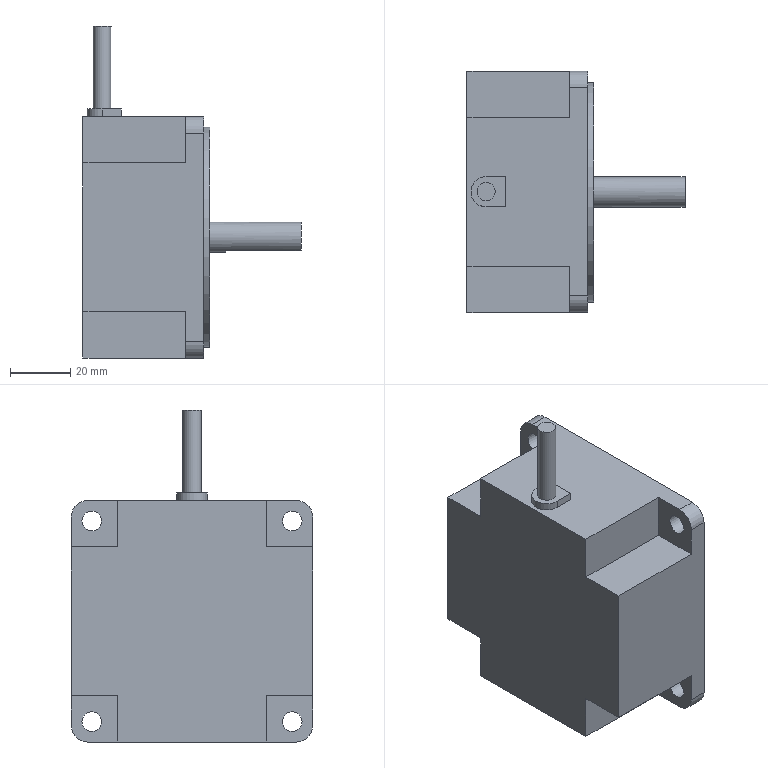Part | NX | features 5003_108_Stepper motor 2 | 1 solid | 41 faces | box 72.25 x 80 x 110 mm | volume 229003 mm3 | plane 28 | cylinder 13 | commonest cylinder face diameters 6.5 x4 11 x4 10 x2 6 x1 35 x1 73 x1
STEP:
#1=CARTESIAN_POINT('',(-49.115,60.,-76.5));
#2=VERTEX_POINT('',#1);
#3=CARTESIAN_POINT('',(-55.415,60.,-76.5));
#4=VERTEX_POINT('',#3);
#5=CARTESIAN_POINT('',(-49.115,60.,-76.5));
#6=DIRECTION('',(-1.,0.,0.));
#7=VECTOR('',#6,1000.);
#8=LINE('',#5,#7);
#9=EDGE_CURVE('',#2,#4,#8,.T.);
#10=ORIENTED_EDGE('',*,*,#9,.T.);
#11=CARTESIAN_POINT('',(-55.415,50.,-76.5));
#12=VERTEX_POINT('',#11);
#13=CARTESIAN_POINT('',(-55.415,55.,-76.5));
#14=DIRECTION('',(0.,0.,1.));
#15=DIRECTION('',(0.,-1.,0.));
#16=AXIS2_PLACEMENT_3D('',#13,#14,#15);
#17=CIRCLE('',#16,5.);
#18=EDGE_CURVE('',#4,#12,#17,.T.);
#19=ORIENTED_EDGE('',*,*,#18,.T.);
#20=CARTESIAN_POINT('',(-49.115,50.,-76.5));
#21=VERTEX_POINT('',#20);
#22=CARTESIAN_POINT('',(-49.115,50.,-76.5));
#23=DIRECTION('',(1.,0.,0.));
#24=VECTOR('',#23,1000.);
#25=LINE('',#22,#24);
#26=EDGE_CURVE('',#12,#21,#25,.T.);
#27=ORIENTED_EDGE('',*,*,#26,.T.);
#28=CARTESIAN_POINT('',(-49.115,60.,-76.5));
#29=DIRECTION('',(0.,1.,0.));
#30=VECTOR('',#29,1000.);
#31=LINE('',#28,#30);
#32=EDGE_CURVE('',#21,#2,#31,.T.);
#33=ORIENTED_EDGE('',*,*,#32,.T.);
#34=EDGE_LOOP('',(#10,#19,#27,#33));
#35=FACE_BOUND('',#34,.T.);
#36=CARTESIAN_POINT('',(-55.415,52.,-76.5));
#37=VERTEX_POINT('',#36);
#38=CARTESIAN_POINT('',(-55.415,55.,-76.5));
#39=DIRECTION('',(0.,0.,1.));
#40=DIRECTION('',(0.,-1.,0.));
#41=AXIS2_PLACEMENT_3D('',#38,#39,#40);
#42=CIRCLE('',#41,3.);
#43=EDGE_CURVE('',#37,#37,#42,.T.);
#44=ORIENTED_EDGE('',*,*,#43,.F.);
#45=EDGE_LOOP('',(#44));
#46=FACE_BOUND('',#45,.T.);
#47=CARTESIAN_POINT('',(-55.415,55.,-76.5));
#48=DIRECTION('',(0.,0.,1.));
#49=DIRECTION('',(0.,-1.,0.));
#50=AXIS2_PLACEMENT_3D('',#47,#48,#49);
#51=PLANE('',#50);
#52=ADVANCED_FACE('',(#35,#46),#51,.T.);
#53=CARTESIAN_POINT('',(-27.725,20.5,-79.));
#54=VERTEX_POINT('',#53);
#55=CARTESIAN_POINT('',(-21.725,20.5,-79.));
#56=VERTEX_POINT('',#55);
#57=CARTESIAN_POINT('',(-61.725,20.5,-79.));
#58=DIRECTION('',(1.,0.,0.));
#59=VECTOR('',#58,1000.);
#60=LINE('',#57,#59);
#61=EDGE_CURVE('',#54,#56,#60,.T.);
#62=ORIENTED_EDGE('',*,*,#61,.T.);
#63=CARTESIAN_POINT('',(-21.725,89.5,-79.));
#64=VERTEX_POINT('',#63);
#65=CARTESIAN_POINT('',(-21.725,95.,-79.));
#66=DIRECTION('',(0.,1.,0.));
#67=VECTOR('',#66,1000.);
#68=LINE('',#65,#67);
#69=EDGE_CURVE('',#56,#64,#68,.T.);
#70=ORIENTED_EDGE('',*,*,#69,.T.);
#71=CARTESIAN_POINT('',(-27.725,89.5,-79.));
#72=VERTEX_POINT('',#71);
#73=CARTESIAN_POINT('',(-61.725,89.5,-79.));
#74=DIRECTION('',(1.,0.,0.));
#75=VECTOR('',#74,1000.);
#76=LINE('',#73,#75);
#77=EDGE_CURVE('',#64,#72,#76,.F.);
#78=ORIENTED_EDGE('',*,*,#77,.T.);
#79=CARTESIAN_POINT('',(-27.725,79.65,-79.));
#80=VERTEX_POINT('',#79);
#81=CARTESIAN_POINT('',(-27.725,95.,-79.));
#82=DIRECTION('',(0.,-1.,0.));
#83=VECTOR('',#82,1000.);
#84=LINE('',#81,#83);
#85=EDGE_CURVE('',#72,#80,#84,.T.);
#86=ORIENTED_EDGE('',*,*,#85,.T.);
#87=CARTESIAN_POINT('',(-61.725,79.65,-79.));
#88=VERTEX_POINT('',#87);
#89=CARTESIAN_POINT('',(-27.725,79.65,-79.));
#90=DIRECTION('',(-1.,0.,0.));
#91=VECTOR('',#90,1000.);
#92=LINE('',#89,#91);
#93=EDGE_CURVE('',#80,#88,#92,.T.);
#94=ORIENTED_EDGE('',*,*,#93,.T.);
#95=CARTESIAN_POINT('',(-61.725,30.35,-79.));
#96=VERTEX_POINT('',#95);
#97=CARTESIAN_POINT('',(-61.725,95.,-79.));
#98=DIRECTION('',(0.,-1.,0.));
#99=VECTOR('',#98,1000.);
#100=LINE('',#97,#99);
#101=EDGE_CURVE('',#88,#96,#100,.T.);
#102=ORIENTED_EDGE('',*,*,#101,.T.);
#103=CARTESIAN_POINT('',(-27.725,30.35,-79.));
#104=VERTEX_POINT('',#103);
#105=CARTESIAN_POINT('',(-27.725,30.35,-79.));
#106=DIRECTION('',(-1.,0.,0.));
#107=VECTOR('',#106,1000.);
#108=LINE('',#105,#107);
#109=EDGE_CURVE('',#104,#96,#108,.T.);
#110=ORIENTED_EDGE('',*,*,#109,.F.);
#111=CARTESIAN_POINT('',(-27.725,95.,-79.));
#112=DIRECTION('',(0.,-1.,0.));
#113=VECTOR('',#112,1000.);
#114=LINE('',#111,#113);
#115=EDGE_CURVE('',#104,#54,#114,.T.);
#116=ORIENTED_EDGE('',*,*,#115,.T.);
#117=EDGE_LOOP('',(#62,#70,#78,#86,#94,#102,#110,#116));
#118=FACE_BOUND('',#117,.T.);
#119=CARTESIAN_POINT('',(-55.415,60.,-79.));
#120=VERTEX_POINT('',#119);
#121=CARTESIAN_POINT('',(-55.415,50.,-79.));
#122=VERTEX_POINT('',#121);
#123=CARTESIAN_POINT('',(-55.415,55.,-79.));
#124=DIRECTION('',(0.,0.,1.));
#125=DIRECTION('',(0.,-1.,0.));
#126=AXIS2_PLACEMENT_3D('',#123,#124,#125);
#127=CIRCLE('',#126,5.);
#128=EDGE_CURVE('',#120,#122,#127,.T.);
#129=ORIENTED_EDGE('',*,*,#128,.F.);
#130=CARTESIAN_POINT('',(-49.115,60.,-79.));
#131=VERTEX_POINT('',#130);
#132=CARTESIAN_POINT('',(-49.115,60.,-79.));
#133=DIRECTION('',(-1.,0.,0.));
#134=VECTOR('',#133,1000.);
#135=LINE('',#132,#134);
#136=EDGE_CURVE('',#131,#120,#135,.T.);
#137=ORIENTED_EDGE('',*,*,#136,.F.);
#138=CARTESIAN_POINT('',(-49.115,50.,-79.));
#139=VERTEX_POINT('',#138);
#140=CARTESIAN_POINT('',(-49.115,60.,-79.));
#141=DIRECTION('',(0.,1.,0.));
#142=VECTOR('',#141,1000.);
#143=LINE('',#140,#142);
#144=EDGE_CURVE('',#139,#131,#143,.T.);
#145=ORIENTED_EDGE('',*,*,#144,.F.);
#146=CARTESIAN_POINT('',(-49.115,50.,-79.));
#147=DIRECTION('',(1.,0.,0.));
#148=VECTOR('',#147,1000.);
#149=LINE('',#146,#148);
#150=EDGE_CURVE('',#122,#139,#149,.T.);
#151=ORIENTED_EDGE('',*,*,#150,.F.);
#152=EDGE_LOOP('',(#129,#137,#145,#151));
#153=FACE_BOUND('',#152,.T.);
#154=CARTESIAN_POINT('',(-61.725,95.,-79.));
#155=DIRECTION('',(0.,0.,1.));
#156=DIRECTION('',(0.,-1.,0.));
#157=AXIS2_PLACEMENT_3D('',#154,#155,#156);
#158=PLANE('',#157);
#159=ADVANCED_FACE('',(#118,#153),#158,.T.);
#160=CARTESIAN_POINT('',(-26.225,37.5,-119.));
#161=VERTEX_POINT('',#160);
#162=CARTESIAN_POINT('',(-26.225,55.,-119.));
#163=DIRECTION('',(1.,0.,0.));
#164=DIRECTION('',(0.,-1.,0.));
#165=AXIS2_PLACEMENT_3D('',#162,#163,#164);
#166=CIRCLE('',#165,17.5);
#167=EDGE_CURVE('',#161,#161,#166,.T.);
#168=ORIENTED_EDGE('',*,*,#167,.T.);
#169=EDGE_LOOP('',(#168));
#170=FACE_BOUND('',#169,.T.);
#171=CARTESIAN_POINT('',(-26.225,50.,-119.));
#172=VERTEX_POINT('',#171);
#173=CARTESIAN_POINT('',(-26.225,55.,-119.));
#174=DIRECTION('',(1.,0.,0.));
#175=DIRECTION('',(0.,-1.,0.));
#176=AXIS2_PLACEMENT_3D('',#173,#174,#175);
#177=CIRCLE('',#176,5.);
#178=EDGE_CURVE('',#172,#172,#177,.T.);
#179=ORIENTED_EDGE('',*,*,#178,.F.);
#180=EDGE_LOOP('',(#179));
#181=FACE_BOUND('',#180,.T.);
#182=CARTESIAN_POINT('',(-26.225,55.,-119.));
#183=DIRECTION('',(1.,0.,0.));
#184=DIRECTION('',(0.,-1.,0.));
#185=AXIS2_PLACEMENT_3D('',#182,#183,#184);
#186=PLANE('',#185);
#187=ADVANCED_FACE('',(#170,#181),#186,.T.);
#188=CARTESIAN_POINT('',(-27.725,95.,-84.5));
#189=VERTEX_POINT('',#188);
#190=CARTESIAN_POINT('',(-21.725,95.,-84.5));
#191=VERTEX_POINT('',#190);
#192=CARTESIAN_POINT('',(-61.725,95.,-84.5));
#193=DIRECTION('',(1.,0.,0.));
#194=VECTOR('',#193,1000.);
#195=LINE('',#192,#194);
#196=EDGE_CURVE('',#189,#191,#195,.T.);
#197=ORIENTED_EDGE('',*,*,#196,.T.);
#198=CARTESIAN_POINT('',(-21.725,95.,-153.5));
#199=VERTEX_POINT('',#198);
#200=CARTESIAN_POINT('',(-21.725,95.,-159.));
#201=DIRECTION('',(0.,0.,-1.));
#202=VECTOR('',#201,1000.);
#203=LINE('',#200,#202);
#204=EDGE_CURVE('',#191,#199,#203,.T.);
#205=ORIENTED_EDGE('',*,*,#204,.T.);
#206=CARTESIAN_POINT('',(-27.725,95.,-153.5));
#207=VERTEX_POINT('',#206);
#208=CARTESIAN_POINT('',(-61.725,95.,-153.5));
#209=DIRECTION('',(1.,0.,0.));
#210=VECTOR('',#209,1000.);
#211=LINE('',#208,#210);
#212=EDGE_CURVE('',#199,#207,#211,.F.);
#213=ORIENTED_EDGE('',*,*,#212,.T.);
#214=CARTESIAN_POINT('',(-27.725,95.,-143.65));
#215=VERTEX_POINT('',#214);
#216=CARTESIAN_POINT('',(-27.725,95.,-159.));
#217=DIRECTION('',(0.,0.,1.));
#218=VECTOR('',#217,1000.);
#219=LINE('',#216,#218);
#220=EDGE_CURVE('',#207,#215,#219,.T.);
#221=ORIENTED_EDGE('',*,*,#220,.T.);
#222=CARTESIAN_POINT('',(-61.725,95.,-143.65));
#223=VERTEX_POINT('',#222);
#224=CARTESIAN_POINT('',(-27.725,95.,-143.65));
#225=DIRECTION('',(-1.,0.,0.));
#226=VECTOR('',#225,1000.);
#227=LINE('',#224,#226);
#228=EDGE_CURVE('',#215,#223,#227,.T.);
#229=ORIENTED_EDGE('',*,*,#228,.T.);
#230=CARTESIAN_POINT('',(-61.725,95.,-94.35));
#231=VERTEX_POINT('',#230);
#232=CARTESIAN_POINT('',(-61.725,95.,-159.));
#233=DIRECTION('',(0.,0.,1.));
#234=VECTOR('',#233,1000.);
#235=LINE('',#232,#234);
#236=EDGE_CURVE('',#223,#231,#235,.T.);
#237=ORIENTED_EDGE('',*,*,#236,.T.);
#238=CARTESIAN_POINT('',(-27.725,95.,-94.35));
#239=VERTEX_POINT('',#238);
#240=CARTESIAN_POINT('',(-27.725,95.,-94.35));
#241=DIRECTION('',(-1.,0.,0.));
#242=VECTOR('',#241,1000.);
#243=LINE('',#240,#242);
#244=EDGE_CURVE('',#239,#231,#243,.T.);
#245=ORIENTED_EDGE('',*,*,#244,.F.);
#246=CARTESIAN_POINT('',(-27.725,95.,-159.));
#247=DIRECTION('',(0.,0.,1.));
#248=VECTOR('',#247,1000.);
#249=LINE('',#246,#248);
#250=EDGE_CURVE('',#239,#189,#249,.T.);
#251=ORIENTED_EDGE('',*,*,#250,.T.);
#252=EDGE_LOOP('',(#197,#205,#213,#221,#229,#237,#245,#251));
#253=FACE_BOUND('',#252,.T.);
#254=CARTESIAN_POINT('',(-61.725,95.,-159.));
#255=DIRECTION('',(0.,1.,0.));
#256=DIRECTION('',(0.,0.,1.));
#257=AXIS2_PLACEMENT_3D('',#254,#255,#256);
#258=PLANE('',#257);
#259=ADVANCED_FACE('',(#253),#258,.T.);
#260=CARTESIAN_POINT('',(-27.725,89.5,-159.));
#261=VERTEX_POINT('',#260);
#262=CARTESIAN_POINT('',(-21.725,89.5,-159.));
#263=VERTEX_POINT('',#262);
#264=CARTESIAN_POINT('',(-61.725,89.5,-159.));
#265=DIRECTION('',(1.,0.,0.));
#266=VECTOR('',#265,1000.);
#267=LINE('',#264,#266);
#268=EDGE_CURVE('',#261,#263,#267,.T.);
#269=ORIENTED_EDGE('',*,*,#268,.T.);
#270=CARTESIAN_POINT('',(-21.725,20.5,-159.));
#271=VERTEX_POINT('',#270);
#272=CARTESIAN_POINT('',(-21.725,95.,-159.));
#273=DIRECTION('',(0.,-1.,0.));
#274=VECTOR('',#273,1000.);
#275=LINE('',#272,#274);
#276=EDGE_CURVE('',#263,#271,#275,.T.);
#277=ORIENTED_EDGE('',*,*,#276,.T.);
#278=CARTESIAN_POINT('',(-27.725,20.5,-159.));
#279=VERTEX_POINT('',#278);
#280=CARTESIAN_POINT('',(-61.725,20.5,-159.));
#281=DIRECTION('',(1.,0.,0.));
#282=VECTOR('',#281,1000.);
#283=LINE('',#280,#282);
#284=EDGE_CURVE('',#271,#279,#283,.F.);
#285=ORIENTED_EDGE('',*,*,#284,.T.);
#286=CARTESIAN_POINT('',(-27.725,30.35,-159.));
#287=VERTEX_POINT('',#286);
#288=CARTESIAN_POINT('',(-27.725,95.,-159.));
#289=DIRECTION('',(0.,1.,0.));
#290=VECTOR('',#289,1000.);
#291=LINE('',#288,#290);
#292=EDGE_CURVE('',#279,#287,#291,.T.);
#293=ORIENTED_EDGE('',*,*,#292,.T.);
#294=CARTESIAN_POINT('',(-61.725,30.35,-159.));
#295=VERTEX_POINT('',#294);
#296=CARTESIAN_POINT('',(-27.725,30.35,-159.));
#297=DIRECTION('',(-1.,0.,0.));
#298=VECTOR('',#297,1000.);
#299=LINE('',#296,#298);
#300=EDGE_CURVE('',#287,#295,#299,.T.);
#301=ORIENTED_EDGE('',*,*,#300,.T.);
#302=CARTESIAN_POINT('',(-61.725,79.65,-159.));
#303=VERTEX_POINT('',#302);
#304=CARTESIAN_POINT('',(-61.725,95.,-159.));
#305=DIRECTION('',(0.,1.,0.));
#306=VECTOR('',#305,1000.);
#307=LINE('',#304,#306);
#308=EDGE_CURVE('',#295,#303,#307,.T.);
#309=ORIENTED_EDGE('',*,*,#308,.T.);
#310=CARTESIAN_POINT('',(-27.725,79.65,-159.));
#311=VERTEX_POINT('',#310);
#312=CARTESIAN_POINT('',(-27.725,79.65,-159.));
#313=DIRECTION('',(-1.,0.,0.));
#314=VECTOR('',#313,1000.);
#315=LINE('',#312,#314);
#316=EDGE_CURVE('',#311,#303,#315,.T.);
#317=ORIENTED_EDGE('',*,*,#316,.F.);
#318=CARTESIAN_POINT('',(-27.725,95.,-159.));
#319=DIRECTION('',(0.,1.,0.));
#320=VECTOR('',#319,1000.);
#321=LINE('',#318,#320);
#322=EDGE_CURVE('',#311,#261,#321,.T.);
#323=ORIENTED_EDGE('',*,*,#322,.T.);
#324=EDGE_LOOP('',(#269,#277,#285,#293,#301,#309,#317,#323));
#325=FACE_BOUND('',#324,.T.);
#326=CARTESIAN_POINT('',(-61.725,95.,-159.));
#327=DIRECTION('',(0.,0.,-1.));
#328=DIRECTION('',(0.,1.,0.));
#329=AXIS2_PLACEMENT_3D('',#326,#327,#328);
#330=PLANE('',#329);
#331=ADVANCED_FACE('',(#325),#330,.T.);
#332=CARTESIAN_POINT('',(-27.725,15.,-153.5));
#333=VERTEX_POINT('',#332);
#334=CARTESIAN_POINT('',(-21.725,15.,-153.5));
#335=VERTEX_POINT('',#334);
#336=CARTESIAN_POINT('',(-61.725,15.,-153.5));
#337=DIRECTION('',(1.,0.,0.));
#338=VECTOR('',#337,1000.);
#339=LINE('',#336,#338);
#340=EDGE_CURVE('',#333,#335,#339,.T.);
#341=ORIENTED_EDGE('',*,*,#340,.T.);
#342=CARTESIAN_POINT('',(-21.725,15.,-84.5));
#343=VERTEX_POINT('',#342);
#344=CARTESIAN_POINT('',(-21.725,15.,-159.));
#345=DIRECTION('',(0.,0.,1.));
#346=VECTOR('',#345,1000.);
#347=LINE('',#344,#346);
#348=EDGE_CURVE('',#335,#343,#347,.T.);
#349=ORIENTED_EDGE('',*,*,#348,.T.);
#350=CARTESIAN_POINT('',(-27.725,15.,-84.5));
#351=VERTEX_POINT('',#350);
#352=CARTESIAN_POINT('',(-61.725,15.,-84.5));
#353=DIRECTION('',(1.,0.,0.));
#354=VECTOR('',#353,1000.);
#355=LINE('',#352,#354);
#356=EDGE_CURVE('',#343,#351,#355,.F.);
#357=ORIENTED_EDGE('',*,*,#356,.T.);
#358=CARTESIAN_POINT('',(-27.725,15.,-94.35));
#359=VERTEX_POINT('',#358);
#360=CARTESIAN_POINT('',(-27.725,15.,-159.));
#361=DIRECTION('',(0.,0.,-1.));
#362=VECTOR('',#361,1000.);
#363=LINE('',#360,#362);
#364=EDGE_CURVE('',#351,#359,#363,.T.);
#365=ORIENTED_EDGE('',*,*,#364,.T.);
#366=CARTESIAN_POINT('',(-61.725,15.,-94.35));
#367=VERTEX_POINT('',#366);
#368=CARTESIAN_POINT('',(-27.725,15.,-94.35));
#369=DIRECTION('',(-1.,0.,0.));
#370=VECTOR('',#369,1000.);
#371=LINE('',#368,#370);
#372=EDGE_CURVE('',#359,#367,#371,.T.);
#373=ORIENTED_EDGE('',*,*,#372,.T.);
#374=CARTESIAN_POINT('',(-61.725,15.,-143.65));
#375=VERTEX_POINT('',#374);
#376=CARTESIAN_POINT('',(-61.725,15.,-159.));
#377=DIRECTION('',(0.,0.,-1.));
#378=VECTOR('',#377,1000.);
#379=LINE('',#376,#378);
#380=EDGE_CURVE('',#367,#375,#379,.T.);
#381=ORIENTED_EDGE('',*,*,#380,.T.);
#382=CARTESIAN_POINT('',(-27.725,15.,-143.65));
#383=VERTEX_POINT('',#382);
#384=CARTESIAN_POINT('',(-27.725,15.,-143.65));
#385=DIRECTION('',(-1.,0.,0.));
#386=VECTOR('',#385,1000.);
#387=LINE('',#384,#386);
#388=EDGE_CURVE('',#383,#375,#387,.T.);
#389=ORIENTED_EDGE('',*,*,#388,.F.);
#390=CARTESIAN_POINT('',(-27.725,15.,-159.));
#391=DIRECTION('',(0.,0.,-1.));
#392=VECTOR('',#391,1000.);
#393=LINE('',#390,#392);
#394=EDGE_CURVE('',#383,#333,#393,.T.);
#395=ORIENTED_EDGE('',*,*,#394,.T.);
#396=EDGE_LOOP('',(#341,#349,#357,#365,#373,#381,#389,#395));
#397=FACE_BOUND('',#396,.T.);
#398=CARTESIAN_POINT('',(-61.725,15.,-159.));
#399=DIRECTION('',(0.,-1.,0.));
#400=DIRECTION('',(0.,0.,-1.));
#401=AXIS2_PLACEMENT_3D('',#398,#399,#400);
#402=PLANE('',#401);
#403=ADVANCED_FACE('',(#397),#402,.T.);
#404=ORIENTED_EDGE('',*,*,#356,.F.);
#405=CARTESIAN_POINT('',(-21.725,20.5,-84.5));
#406=DIRECTION('',(1.,0.,0.));
#407=DIRECTION('',(0.,-1.,0.));
#408=AXIS2_PLACEMENT_3D('',#405,#406,#407);
#409=CIRCLE('',#408,5.5);
#410=EDGE_CURVE('',#343,#56,#409,.F.);
#411=ORIENTED_EDGE('',*,*,#410,.T.);
#412=ORIENTED_EDGE('',*,*,#61,.F.);
#413=CARTESIAN_POINT('',(-27.725,20.5,-84.5));
#414=DIRECTION('',(-1.,0.,0.));
#415=DIRECTION('',(0.,1.,0.));
#416=AXIS2_PLACEMENT_3D('',#413,#414,#415);
#417=CIRCLE('',#416,5.5);
#418=EDGE_CURVE('',#351,#54,#417,.T.);
#419=ORIENTED_EDGE('',*,*,#418,.F.);
#420=EDGE_LOOP('',(#404,#411,#412,#419));
#421=FACE_BOUND('',#420,.T.);
#422=CARTESIAN_POINT('',(-61.725,20.5,-84.5));
#423=DIRECTION('',(1.,0.,0.));
#424=DIRECTION('',(0.,-1.,0.));
#425=AXIS2_PLACEMENT_3D('',#422,#423,#424);
#426=CYLINDRICAL_SURFACE('',#425,5.5);
#427=ADVANCED_FACE('',(#421),#426,.T.);
#428=ORIENTED_EDGE('',*,*,#77,.F.);
#429=CARTESIAN_POINT('',(-21.725,89.5,-84.5));
#430=DIRECTION('',(1.,0.,0.));
#431=DIRECTION('',(0.,-1.,0.));
#432=AXIS2_PLACEMENT_3D('',#429,#430,#431);
#433=CIRCLE('',#432,5.5);
#434=EDGE_CURVE('',#64,#191,#433,.F.);
#435=ORIENTED_EDGE('',*,*,#434,.T.);
#436=ORIENTED_EDGE('',*,*,#196,.F.);
#437=CARTESIAN_POINT('',(-27.725,89.5,-84.5));
#438=DIRECTION('',(-1.,0.,0.));
#439=DIRECTION('',(0.,1.,0.));
#440=AXIS2_PLACEMENT_3D('',#437,#438,#439);
#441=CIRCLE('',#440,5.5);
#442=EDGE_CURVE('',#72,#189,#441,.T.);
#443=ORIENTED_EDGE('',*,*,#442,.F.);
#444=EDGE_LOOP('',(#428,#435,#436,#443));
#445=FACE_BOUND('',#444,.T.);
#446=CARTESIAN_POINT('',(-61.725,89.5,-84.5));
#447=DIRECTION('',(1.,0.,0.));
#448=DIRECTION('',(0.,-1.,0.));
#449=AXIS2_PLACEMENT_3D('',#446,#447,#448);
#450=CYLINDRICAL_SURFACE('',#449,5.5);
#451=ADVANCED_FACE('',(#445),#450,.T.);
#452=ORIENTED_EDGE('',*,*,#212,.F.);
#453=CARTESIAN_POINT('',(-21.725,89.5,-153.5));
#454=DIRECTION('',(1.,0.,0.));
#455=DIRECTION('',(0.,-1.,0.));
#456=AXIS2_PLACEMENT_3D('',#453,#454,#455);
#457=CIRCLE('',#456,5.5);
#458=EDGE_CURVE('',#199,#263,#457,.F.);
#459=ORIENTED_EDGE('',*,*,#458,.T.);
#460=ORIENTED_EDGE('',*,*,#268,.F.);
#461=CARTESIAN_POINT('',(-27.725,89.5,-153.5));
#462=DIRECTION('',(-1.,0.,0.));
#463=DIRECTION('',(0.,1.,0.));
#464=AXIS2_PLACEMENT_3D('',#461,#462,#463);
#465=CIRCLE('',#464,5.5);
#466=EDGE_CURVE('',#207,#261,#465,.T.);
#467=ORIENTED_EDGE('',*,*,#466,.F.);
#468=EDGE_LOOP('',(#452,#459,#460,#467));
#469=FACE_BOUND('',#468,.T.);
#470=CARTESIAN_POINT('',(-61.725,89.5,-153.5));
#471=DIRECTION('',(1.,0.,0.));
#472=DIRECTION('',(0.,-1.,0.));
#473=AXIS2_PLACEMENT_3D('',#470,#471,#472);
#474=CYLINDRICAL_SURFACE('',#473,5.5);
#475=ADVANCED_FACE('',(#469),#474,.T.);
#476=ORIENTED_EDGE('',*,*,#284,.F.);
#477=CARTESIAN_POINT('',(-21.725,20.5,-153.5));
#478=DIRECTION('',(1.,0.,0.));
#479=DIRECTION('',(0.,-1.,0.));
#480=AXIS2_PLACEMENT_3D('',#477,#478,#479);
#481=CIRCLE('',#480,5.5);
#482=EDGE_CURVE('',#271,#335,#481,.F.);
#483=ORIENTED_EDGE('',*,*,#482,.T.);
#484=ORIENTED_EDGE('',*,*,#340,.F.);
#485=CARTESIAN_POINT('',(-27.725,20.5,-153.5));
#486=DIRECTION('',(-1.,0.,0.));
#487=DIRECTION('',(0.,1.,0.));
#488=AXIS2_PLACEMENT_3D('',#485,#486,#487);
#489=CIRCLE('',#488,5.5);
#490=EDGE_CURVE('',#279,#333,#489,.T.);
#491=ORIENTED_EDGE('',*,*,#490,.F.);
#492=EDGE_LOOP('',(#476,#483,#484,#491));
#493=FACE_BOUND('',#492,.T.);
#494=CARTESIAN_POINT('',(-61.725,20.5,-153.5));
#495=DIRECTION('',(1.,0.,0.));
#496=DIRECTION('',(0.,-1.,0.));
#497=AXIS2_PLACEMENT_3D('',#494,#495,#496);
#498=CYLINDRICAL_SURFACE('',#497,5.5);
#499=ADVANCED_FACE('',(#493),#498,.T.);
#500=CARTESIAN_POINT('',(-27.725,91.484,-85.766));
#501=VERTEX_POINT('',#500);
#502=CARTESIAN_POINT('',(-27.725,88.234,-85.766));
#503=DIRECTION('',(-1.,0.,0.));
#504=DIRECTION('',(0.,1.,0.));
#505=AXIS2_PLACEMENT_3D('',#502,#503,#504);
#506=CIRCLE('',#505,3.25);
#507=EDGE_CURVE('',#501,#501,#506,.T.);
#508=ORIENTED_EDGE('',*,*,#507,.T.);
#509=EDGE_LOOP('',(#508));
#510=FACE_BOUND('',#509,.T.);
#511=CARTESIAN_POINT('',(-21.725,84.984,-85.766));
#512=VERTEX_POINT('',#511);
#513=CARTESIAN_POINT('',(-21.725,88.234,-85.766));
#514=DIRECTION('',(1.,0.,0.));
#515=DIRECTION('',(0.,-1.,0.));
#516=AXIS2_PLACEMENT_3D('',#513,#514,#515);
#517=CIRCLE('',#516,3.25);
#518=EDGE_CURVE('',#512,#512,#517,.F.);
#519=ORIENTED_EDGE('',*,*,#518,.F.);
#520=EDGE_LOOP('',(#519));
#521=FACE_BOUND('',#520,.T.);
#522=CARTESIAN_POINT('',(-19.725,88.234,-85.766));
#523=DIRECTION('',(1.,0.,0.));
#524=DIRECTION('',(0.,-1.,0.));
#525=AXIS2_PLACEMENT_3D('',#522,#523,#524);
#526=CYLINDRICAL_SURFACE('',#525,3.25);
#527=ADVANCED_FACE('',(#510,#521),#526,.F.);
#528=CARTESIAN_POINT('',(-27.725,25.016,-85.766));
#529=VERTEX_POINT('',#528);
#530=CARTESIAN_POINT('',(-27.725,21.766,-85.766));
#531=DIRECTION('',(-1.,0.,0.));
#532=DIRECTION('',(0.,1.,0.));
#533=AXIS2_PLACEMENT_3D('',#530,#531,#532);
#534=CIRCLE('',#533,3.25);
#535=EDGE_CURVE('',#529,#529,#534,.T.);
#536=ORIENTED_EDGE('',*,*,#535,.T.);
#537=EDGE_LOOP('',(#536));
#538=FACE_BOUND('',#537,.T.);
#539=CARTESIAN_POINT('',(-21.725,18.516,-85.766));
#540=VERTEX_POINT('',#539);
#541=CARTESIAN_POINT('',(-21.725,21.766,-85.766));
#542=DIRECTION('',(1.,0.,0.));
#543=DIRECTION('',(0.,-1.,0.));
#544=AXIS2_PLACEMENT_3D('',#541,#542,#543);
#545=CIRCLE('',#544,3.25);
#546=EDGE_CURVE('',#540,#540,#545,.F.);
#547=ORIENTED_EDGE('',*,*,#546,.F.);
#548=EDGE_LOOP('',(#547));
#549=FACE_BOUND('',#548,.T.);
#550=CARTESIAN_POINT('',(-19.725,21.766,-85.766));
#551=DIRECTION('',(1.,0.,0.));
#552=DIRECTION('',(0.,-1.,0.));
#553=AXIS2_PLACEMENT_3D('',#550,#551,#552);
#554=CYLINDRICAL_SURFACE('',#553,3.25);
#555=ADVANCED_FACE('',(#538,#549),#554,.F.);
#556=CARTESIAN_POINT('',(-27.725,25.016,-152.234));
#557=VERTEX_POINT('',#556);
#558=CARTESIAN_POINT('',(-27.725,21.766,-152.234));
#559=DIRECTION('',(-1.,0.,0.));
#560=DIRECTION('',(0.,1.,0.));
#561=AXIS2_PLACEMENT_3D('',#558,#559,#560);
#562=CIRCLE('',#561,3.25);
#563=EDGE_CURVE('',#557,#557,#562,.T.);
#564=ORIENTED_EDGE('',*,*,#563,.T.);
#565=EDGE_LOOP('',(#564));
#566=FACE_BOUND('',#565,.T.);
#567=CARTESIAN_POINT('',(-21.725,18.516,-152.234));
#568=VERTEX_POINT('',#567);
#569=CARTESIAN_POINT('',(-21.725,21.766,-152.234));
#570=DIRECTION('',(1.,0.,0.));
#571=DIRECTION('',(0.,-1.,0.));
#572=AXIS2_PLACEMENT_3D('',#569,#570,#571);
#573=CIRCLE('',#572,3.25);
#574=EDGE_CURVE('',#568,#568,#573,.F.);
#575=ORIENTED_EDGE('',*,*,#574,.F.);
#576=EDGE_LOOP('',(#575));
#577=FACE_BOUND('',#576,.T.);
#578=CARTESIAN_POINT('',(-19.725,21.766,-152.234));
#579=DIRECTION('',(1.,0.,0.));
#580=DIRECTION('',(0.,-1.,0.));
#581=AXIS2_PLACEMENT_3D('',#578,#579,#580);
#582=CYLINDRICAL_SURFACE('',#581,3.25);
#583=ADVANCED_FACE('',(#566,#577),#582,.F.);
#584=CARTESIAN_POINT('',(-27.725,91.484,-152.234));
#585=VERTEX_POINT('',#584);
#586=CARTESIAN_POINT('',(-27.725,88.234,-152.234));
#587=DIRECTION('',(-1.,0.,0.));
#588=DIRECTION('',(0.,1.,0.));
#589=AXIS2_PLACEMENT_3D('',#586,#587,#588);
#590=CIRCLE('',#589,3.25);
#591=EDGE_CURVE('',#585,#585,#590,.T.);
#592=ORIENTED_EDGE('',*,*,#591,.T.);
#593=EDGE_LOOP('',(#592));
#594=FACE_BOUND('',#593,.T.);
#595=CARTESIAN_POINT('',(-21.725,84.984,-152.234));
#596=VERTEX_POINT('',#595);
#597=CARTESIAN_POINT('',(-21.725,88.234,-152.234));
#598=DIRECTION('',(1.,0.,0.));
#599=DIRECTION('',(0.,-1.,0.));
#600=AXIS2_PLACEMENT_3D('',#597,#598,#599);
#601=CIRCLE('',#600,3.25);
#602=EDGE_CURVE('',#596,#596,#601,.F.);
#603=ORIENTED_EDGE('',*,*,#602,.F.);
#604=EDGE_LOOP('',(#603));
#605=FACE_BOUND('',#604,.T.);
#606=CARTESIAN_POINT('',(-19.725,88.234,-152.234));
#607=DIRECTION('',(1.,0.,0.));
#608=DIRECTION('',(0.,-1.,0.));
#609=AXIS2_PLACEMENT_3D('',#606,#607,#608);
#610=CYLINDRICAL_SURFACE('',#609,3.25);
#611=ADVANCED_FACE('',(#594,#605),#610,.F.);
#612=CARTESIAN_POINT('',(-61.725,79.65,-143.65));
#613=VERTEX_POINT('',#612);
#614=CARTESIAN_POINT('',(-61.725,79.65,-159.));
#615=DIRECTION('',(0.,0.,-1.));
#616=VECTOR('',#615,1000.);
#617=LINE('',#614,#616);
#618=EDGE_CURVE('',#613,#303,#617,.T.);
#619=ORIENTED_EDGE('',*,*,#618,.T.);
#620=ORIENTED_EDGE('',*,*,#308,.F.);
#621=CARTESIAN_POINT('',(-61.725,30.35,-143.65));
#622=VERTEX_POINT('',#621);
#623=CARTESIAN_POINT('',(-61.725,30.35,-143.65));
#624=DIRECTION('',(0.,0.,1.));
#625=VECTOR('',#624,1000.);
#626=LINE('',#623,#625);
#627=EDGE_CURVE('',#295,#622,#626,.T.);
#628=ORIENTED_EDGE('',*,*,#627,.T.);
#629=CARTESIAN_POINT('',(-61.725,15.,-143.65));
#630=DIRECTION('',(0.,-1.,0.));
#631=VECTOR('',#630,1000.);
#632=LINE('',#629,#631);
#633=EDGE_CURVE('',#622,#375,#632,.T.);
#634=ORIENTED_EDGE('',*,*,#633,.T.);
#635=ORIENTED_EDGE('',*,*,#380,.F.);
#636=CARTESIAN_POINT('',(-61.725,30.35,-94.35));
#637=VERTEX_POINT('',#636);
#638=CARTESIAN_POINT('',(-61.725,30.35,-94.35));
#639=DIRECTION('',(0.,1.,0.));
#640=VECTOR('',#639,1000.);
#641=LINE('',#638,#640);
#642=EDGE_CURVE('',#367,#637,#641,.T.);
#643=ORIENTED_EDGE('',*,*,#642,.T.);
#644=CARTESIAN_POINT('',(-61.725,30.35,-79.));
#645=DIRECTION('',(0.,0.,1.));
#646=VECTOR('',#645,1000.);
#647=LINE('',#644,#646);
#648=EDGE_CURVE('',#637,#96,#647,.T.);
#649=ORIENTED_EDGE('',*,*,#648,.T.);
#650=ORIENTED_EDGE('',*,*,#101,.F.);
#651=CARTESIAN_POINT('',(-61.725,79.65,-94.35));
#652=VERTEX_POINT('',#651);
#653=CARTESIAN_POINT('',(-61.725,79.65,-94.35));
#654=DIRECTION('',(0.,0.,-1.));
#655=VECTOR('',#654,1000.);
#656=LINE('',#653,#655);
#657=EDGE_CURVE('',#88,#652,#656,.T.);
#658=ORIENTED_EDGE('',*,*,#657,.T.);
#659=CARTESIAN_POINT('',(-61.725,95.,-94.35));
#660=DIRECTION('',(0.,1.,0.));
#661=VECTOR('',#660,1000.);
#662=LINE('',#659,#661);
#663=EDGE_CURVE('',#652,#231,#662,.T.);
#664=ORIENTED_EDGE('',*,*,#663,.T.);
#665=ORIENTED_EDGE('',*,*,#236,.F.);
#666=CARTESIAN_POINT('',(-61.725,79.65,-143.65));
#667=DIRECTION('',(0.,-1.,0.));
#668=VECTOR('',#667,1000.);
#669=LINE('',#666,#668);
#670=EDGE_CURVE('',#223,#613,#669,.T.);
#671=ORIENTED_EDGE('',*,*,#670,.T.);
#672=EDGE_LOOP('',(#619,#620,#628,#634,#635,#643,#649,#650,#658,#664,#665,#671));
#673=FACE_BOUND('',#672,.T.);
#674=CARTESIAN_POINT('',(-61.725,55.,-119.));
#675=DIRECTION('',(1.,0.,0.));
#676=DIRECTION('',(0.,-1.,0.));
#677=AXIS2_PLACEMENT_3D('',#674,#675,#676);
#678=PLANE('',#677);
#679=ADVANCED_FACE('',(#673),#678,.F.);
#680=ORIENTED_EDGE('',*,*,#633,.F.);
#681=CARTESIAN_POINT('',(-27.725,30.35,-143.65));
#682=VERTEX_POINT('',#681);
#683=CARTESIAN_POINT('',(-27.725,30.35,-143.65));
#684=DIRECTION('',(-1.,0.,0.));
#685=VECTOR('',#684,1000.);
#686=LINE('',#683,#685);
#687=EDGE_CURVE('',#682,#622,#686,.T.);
#688=ORIENTED_EDGE('',*,*,#687,.F.);
#689=CARTESIAN_POINT('',(-27.725,15.,-143.65));
#690=DIRECTION('',(0.,-1.,0.));
#691=VECTOR('',#690,1000.);
#692=LINE('',#689,#691);
#693=EDGE_CURVE('',#682,#383,#692,.T.);
#694=ORIENTED_EDGE('',*,*,#693,.T.);
#695=ORIENTED_EDGE('',*,*,#388,.T.);
#696=EDGE_LOOP('',(#680,#688,#694,#695));
#697=FACE_BOUND('',#696,.T.);
#698=CARTESIAN_POINT('',(-27.725,15.,-143.65));
#699=DIRECTION('',(0.,0.,-1.));
#700=DIRECTION('',(1.,0.,0.));
#701=AXIS2_PLACEMENT_3D('',#698,#699,#700);
#702=PLANE('',#701);
#703=ADVANCED_FACE('',(#697),#702,.T.);
#704=ORIENTED_EDGE('',*,*,#627,.F.);
#705=ORIENTED_EDGE('',*,*,#300,.F.);
#706=CARTESIAN_POINT('',(-27.725,30.35,-143.65));
#707=DIRECTION('',(0.,0.,1.));
#708=VECTOR('',#707,1000.);
#709=LINE('',#706,#708);
#710=EDGE_CURVE('',#287,#682,#709,.T.);
#711=ORIENTED_EDGE('',*,*,#710,.T.);
#712=ORIENTED_EDGE('',*,*,#687,.T.);
#713=EDGE_LOOP('',(#704,#705,#711,#712));
#714=FACE_BOUND('',#713,.T.);
#715=CARTESIAN_POINT('',(-27.725,30.35,-143.65));
#716=DIRECTION('',(0.,-1.,0.));
#717=DIRECTION('',(-1.,0.,0.));
#718=AXIS2_PLACEMENT_3D('',#715,#716,#717);
#719=PLANE('',#718);
#720=ADVANCED_FACE('',(#714),#719,.T.);
#721=ORIENTED_EDGE('',*,*,#563,.F.);
#722=EDGE_LOOP('',(#721));
#723=FACE_BOUND('',#722,.T.);
#724=ORIENTED_EDGE('',*,*,#292,.F.);
#725=ORIENTED_EDGE('',*,*,#490,.T.);
#726=ORIENTED_EDGE('',*,*,#394,.F.);
#727=ORIENTED_EDGE('',*,*,#693,.F.);
#728=ORIENTED_EDGE('',*,*,#710,.F.);
#729=EDGE_LOOP('',(#724,#725,#726,#727,#728));
#730=FACE_BOUND('',#729,.T.);
#731=CARTESIAN_POINT('',(-27.725,55.,-119.));
#732=DIRECTION('',(-1.,0.,0.));
#733=DIRECTION('',(0.,1.,0.));
#734=AXIS2_PLACEMENT_3D('',#731,#732,#733);
#735=PLANE('',#734);
#736=ADVANCED_FACE('',(#723,#730),#735,.T.);
#737=ORIENTED_EDGE('',*,*,#642,.F.);
#738=ORIENTED_EDGE('',*,*,#372,.F.);
#739=CARTESIAN_POINT('',(-27.725,30.35,-94.35));
#740=VERTEX_POINT('',#739);
#741=CARTESIAN_POINT('',(-27.725,30.35,-94.35));
#742=DIRECTION('',(0.,1.,0.));
#743=VECTOR('',#742,1000.);
#744=LINE('',#741,#743);
#745=EDGE_CURVE('',#359,#740,#744,.T.);
#746=ORIENTED_EDGE('',*,*,#745,.T.);
#747=CARTESIAN_POINT('',(-27.725,30.35,-94.35));
#748=DIRECTION('',(-1.,0.,0.));
#749=VECTOR('',#748,1000.);
#750=LINE('',#747,#749);
#751=EDGE_CURVE('',#740,#637,#750,.T.);
#752=ORIENTED_EDGE('',*,*,#751,.T.);
#753=EDGE_LOOP('',(#737,#738,#746,#752));
#754=FACE_BOUND('',#753,.T.);
#755=CARTESIAN_POINT('',(-27.725,30.35,-94.35));
#756=DIRECTION('',(0.,0.,1.));
#757=DIRECTION('',(-1.,0.,0.));
#758=AXIS2_PLACEMENT_3D('',#755,#756,#757);
#759=PLANE('',#758);
#760=ADVANCED_FACE('',(#754),#759,.T.);
#761=ORIENTED_EDGE('',*,*,#648,.F.);
#762=ORIENTED_EDGE('',*,*,#751,.F.);
#763=CARTESIAN_POINT('',(-27.725,30.35,-79.));
#764=DIRECTION('',(0.,0.,1.));
#765=VECTOR('',#764,1000.);
#766=LINE('',#763,#765);
#767=EDGE_CURVE('',#740,#104,#766,.T.);
#768=ORIENTED_EDGE('',*,*,#767,.T.);
#769=ORIENTED_EDGE('',*,*,#109,.T.);
#770=EDGE_LOOP('',(#761,#762,#768,#769));
#771=FACE_BOUND('',#770,.T.);
#772=CARTESIAN_POINT('',(-27.725,30.35,-79.));
#773=DIRECTION('',(0.,-1.,0.));
#774=DIRECTION('',(0.,0.,-1.));
#775=AXIS2_PLACEMENT_3D('',#772,#773,#774);
#776=PLANE('',#775);
#777=ADVANCED_FACE('',(#771),#776,.T.);
#778=ORIENTED_EDGE('',*,*,#535,.F.);
#779=EDGE_LOOP('',(#778));
#780=FACE_BOUND('',#779,.T.);
#781=ORIENTED_EDGE('',*,*,#364,.F.);
#782=ORIENTED_EDGE('',*,*,#418,.T.);
#783=ORIENTED_EDGE('',*,*,#115,.F.);
#784=ORIENTED_EDGE('',*,*,#767,.F.);
#785=ORIENTED_EDGE('',*,*,#745,.F.);
#786=EDGE_LOOP('',(#781,#782,#783,#784,#785));
#787=FACE_BOUND('',#786,.T.);
#788=CARTESIAN_POINT('',(-27.725,55.,-119.));
#789=DIRECTION('',(-1.,0.,0.));
#790=DIRECTION('',(0.,1.,0.));
#791=AXIS2_PLACEMENT_3D('',#788,#789,#790);
#792=PLANE('',#791);
#793=ADVANCED_FACE('',(#780,#787),#792,.T.);
#794=ORIENTED_EDGE('',*,*,#657,.F.);
#795=ORIENTED_EDGE('',*,*,#93,.F.);
#796=CARTESIAN_POINT('',(-27.725,79.65,-94.35));
#797=VERTEX_POINT('',#796);
#798=CARTESIAN_POINT('',(-27.725,79.65,-94.35));
#799=DIRECTION('',(0.,0.,-1.));
#800=VECTOR('',#799,1000.);
#801=LINE('',#798,#800);
#802=EDGE_CURVE('',#80,#797,#801,.T.);
#803=ORIENTED_EDGE('',*,*,#802,.T.);
#804=CARTESIAN_POINT('',(-27.725,79.65,-94.35));
#805=DIRECTION('',(-1.,0.,0.));
#806=VECTOR('',#805,1000.);
#807=LINE('',#804,#806);
#808=EDGE_CURVE('',#797,#652,#807,.T.);
#809=ORIENTED_EDGE('',*,*,#808,.T.);
#810=EDGE_LOOP('',(#794,#795,#803,#809));
#811=FACE_BOUND('',#810,.T.);
#812=CARTESIAN_POINT('',(-27.725,79.65,-94.35));
#813=DIRECTION('',(0.,1.,0.));
#814=DIRECTION('',(0.,0.,1.));
#815=AXIS2_PLACEMENT_3D('',#812,#813,#814);
#816=PLANE('',#815);
#817=ADVANCED_FACE('',(#811),#816,.T.);
#818=ORIENTED_EDGE('',*,*,#663,.F.);
#819=ORIENTED_EDGE('',*,*,#808,.F.);
#820=CARTESIAN_POINT('',(-27.725,95.,-94.35));
#821=DIRECTION('',(0.,1.,0.));
#822=VECTOR('',#821,1000.);
#823=LINE('',#820,#822);
#824=EDGE_CURVE('',#797,#239,#823,.T.);
#825=ORIENTED_EDGE('',*,*,#824,.T.);
#826=ORIENTED_EDGE('',*,*,#244,.T.);
#827=EDGE_LOOP('',(#818,#819,#825,#826));
#828=FACE_BOUND('',#827,.T.);
#829=CARTESIAN_POINT('',(-27.725,95.,-94.35));
#830=DIRECTION('',(0.,0.,1.));
#831=DIRECTION('',(-1.,0.,0.));
#832=AXIS2_PLACEMENT_3D('',#829,#830,#831);
#833=PLANE('',#832);
#834=ADVANCED_FACE('',(#828),#833,.T.);
#835=ORIENTED_EDGE('',*,*,#507,.F.);
#836=EDGE_LOOP('',(#835));
#837=FACE_BOUND('',#836,.T.);
#838=ORIENTED_EDGE('',*,*,#85,.F.);
#839=ORIENTED_EDGE('',*,*,#442,.T.);
#840=ORIENTED_EDGE('',*,*,#250,.F.);
#841=ORIENTED_EDGE('',*,*,#824,.F.);
#842=ORIENTED_EDGE('',*,*,#802,.F.);
#843=EDGE_LOOP('',(#838,#839,#840,#841,#842));
#844=FACE_BOUND('',#843,.T.);
#845=CARTESIAN_POINT('',(-27.725,55.,-119.));
#846=DIRECTION('',(-1.,0.,0.));
#847=DIRECTION('',(0.,1.,0.));
#848=AXIS2_PLACEMENT_3D('',#845,#846,#847);
#849=PLANE('',#848);
#850=ADVANCED_FACE('',(#837,#844),#849,.T.);
#851=ORIENTED_EDGE('',*,*,#591,.F.);
#852=EDGE_LOOP('',(#851));
#853=FACE_BOUND('',#852,.T.);
#854=ORIENTED_EDGE('',*,*,#220,.F.);
#855=ORIENTED_EDGE('',*,*,#466,.T.);
#856=ORIENTED_EDGE('',*,*,#322,.F.);
#857=CARTESIAN_POINT('',(-27.725,79.65,-143.65));
#858=VERTEX_POINT('',#857);
#859=CARTESIAN_POINT('',(-27.725,79.65,-159.));
#860=DIRECTION('',(0.,0.,-1.));
#861=VECTOR('',#860,1000.);
#862=LINE('',#859,#861);
#863=EDGE_CURVE('',#858,#311,#862,.T.);
#864=ORIENTED_EDGE('',*,*,#863,.F.);
#865=CARTESIAN_POINT('',(-27.725,79.65,-143.65));
#866=DIRECTION('',(0.,-1.,0.));
#867=VECTOR('',#866,1000.);
#868=LINE('',#865,#867);
#869=EDGE_CURVE('',#215,#858,#868,.T.);
#870=ORIENTED_EDGE('',*,*,#869,.F.);
#871=EDGE_LOOP('',(#854,#855,#856,#864,#870));
#872=FACE_BOUND('',#871,.T.);
#873=CARTESIAN_POINT('',(-27.725,55.,-119.));
#874=DIRECTION('',(-1.,0.,0.));
#875=DIRECTION('',(0.,1.,0.));
#876=AXIS2_PLACEMENT_3D('',#873,#874,#875);
#877=PLANE('',#876);
#878=ADVANCED_FACE('',(#853,#872),#877,.T.);
#879=ORIENTED_EDGE('',*,*,#618,.F.);
#880=CARTESIAN_POINT('',(-27.725,79.65,-143.65));
#881=DIRECTION('',(-1.,0.,0.));
#882=VECTOR('',#881,1000.);
#883=LINE('',#880,#882);
#884=EDGE_CURVE('',#858,#613,#883,.T.);
#885=ORIENTED_EDGE('',*,*,#884,.F.);
#886=ORIENTED_EDGE('',*,*,#863,.T.);
#887=ORIENTED_EDGE('',*,*,#316,.T.);
#888=EDGE_LOOP('',(#879,#885,#886,#887));
#889=FACE_BOUND('',#888,.T.);
#890=CARTESIAN_POINT('',(-27.725,79.65,-159.));
#891=DIRECTION('',(0.,1.,0.));
#892=DIRECTION('',(1.,0.,0.));
#893=AXIS2_PLACEMENT_3D('',#890,#891,#892);
#894=PLANE('',#893);
#895=ADVANCED_FACE('',(#889),#894,.T.);
#896=ORIENTED_EDGE('',*,*,#670,.F.);
#897=ORIENTED_EDGE('',*,*,#228,.F.);
#898=ORIENTED_EDGE('',*,*,#869,.T.);
#899=ORIENTED_EDGE('',*,*,#884,.T.);
#900=EDGE_LOOP('',(#896,#897,#898,#899));
#901=FACE_BOUND('',#900,.T.);
#902=CARTESIAN_POINT('',(-27.725,79.65,-143.65));
#903=DIRECTION('',(0.,0.,-1.));
#904=DIRECTION('',(1.,0.,0.));
#905=AXIS2_PLACEMENT_3D('',#902,#903,#904);
#906=PLANE('',#905);
#907=ADVANCED_FACE('',(#901),#906,.T.);
#908=ORIENTED_EDGE('',*,*,#69,.F.);
#909=ORIENTED_EDGE('',*,*,#410,.F.);
#910=ORIENTED_EDGE('',*,*,#348,.F.);
#911=ORIENTED_EDGE('',*,*,#482,.F.);
#912=ORIENTED_EDGE('',*,*,#276,.F.);
#913=ORIENTED_EDGE('',*,*,#458,.F.);
#914=ORIENTED_EDGE('',*,*,#204,.F.);
#915=ORIENTED_EDGE('',*,*,#434,.F.);
#916=EDGE_LOOP('',(#908,#909,#910,#911,#912,#913,#914,#915));
#917=FACE_BOUND('',#916,.T.);
#918=CARTESIAN_POINT('',(-21.725,18.5,-119.));
#919=VERTEX_POINT('',#918);
#920=CARTESIAN_POINT('',(-21.725,55.,-119.));
#921=DIRECTION('',(1.,0.,0.));
#922=DIRECTION('',(0.,-1.,0.));
#923=AXIS2_PLACEMENT_3D('',#920,#921,#922);
#924=CIRCLE('',#923,36.5);
#925=EDGE_CURVE('',#919,#919,#924,.T.);
#926=ORIENTED_EDGE('',*,*,#925,.F.);
#927=EDGE_LOOP('',(#926));
#928=FACE_BOUND('',#927,.T.);
#929=ORIENTED_EDGE('',*,*,#602,.T.);
#930=EDGE_LOOP('',(#929));
#931=FACE_BOUND('',#930,.T.);
#932=ORIENTED_EDGE('',*,*,#574,.T.);
#933=EDGE_LOOP('',(#932));
#934=FACE_BOUND('',#933,.T.);
#935=ORIENTED_EDGE('',*,*,#546,.T.);
#936=EDGE_LOOP('',(#935));
#937=FACE_BOUND('',#936,.T.);
#938=ORIENTED_EDGE('',*,*,#518,.T.);
#939=EDGE_LOOP('',(#938));
#940=FACE_BOUND('',#939,.T.);
#941=CARTESIAN_POINT('',(-21.725,55.,-119.));
#942=DIRECTION('',(1.,0.,0.));
#943=DIRECTION('',(0.,-1.,0.));
#944=AXIS2_PLACEMENT_3D('',#941,#942,#943);
#945=PLANE('',#944);
#946=ADVANCED_FACE('',(#917,#928,#931,#934,#937,#940),#945,.T.);
#947=ORIENTED_EDGE('',*,*,#925,.T.);
#948=EDGE_LOOP('',(#947));
#949=FACE_BOUND('',#948,.T.);
#950=CARTESIAN_POINT('',(-19.725,18.5,-119.));
#951=VERTEX_POINT('',#950);
#952=CARTESIAN_POINT('',(-19.725,55.,-119.));
#953=DIRECTION('',(1.,0.,0.));
#954=DIRECTION('',(0.,-1.,0.));
#955=AXIS2_PLACEMENT_3D('',#952,#953,#954);
#956=CIRCLE('',#955,36.5);
#957=EDGE_CURVE('',#951,#951,#956,.T.);
#958=ORIENTED_EDGE('',*,*,#957,.F.);
#959=EDGE_LOOP('',(#958));
#960=FACE_BOUND('',#959,.T.);
#961=CARTESIAN_POINT('',(-21.725,55.,-119.));
#962=DIRECTION('',(1.,0.,0.));
#963=DIRECTION('',(0.,-1.,0.));
#964=AXIS2_PLACEMENT_3D('',#961,#962,#963);
#965=CYLINDRICAL_SURFACE('',#964,36.5);
#966=ADVANCED_FACE('',(#949,#960),#965,.T.);
#967=CARTESIAN_POINT('',(-19.725,37.5,-119.));
#968=VERTEX_POINT('',#967);
#969=CARTESIAN_POINT('',(-19.725,55.,-119.));
#970=DIRECTION('',(1.,0.,0.));
#971=DIRECTION('',(0.,-1.,0.));
#972=AXIS2_PLACEMENT_3D('',#969,#970,#971);
#973=CIRCLE('',#972,17.5);
#974=EDGE_CURVE('',#968,#968,#973,.T.);
#975=ORIENTED_EDGE('',*,*,#974,.F.);
#976=EDGE_LOOP('',(#975));
#977=FACE_BOUND('',#976,.T.);
#978=ORIENTED_EDGE('',*,*,#957,.T.);
#979=EDGE_LOOP('',(#978));
#980=FACE_BOUND('',#979,.T.);
#981=CARTESIAN_POINT('',(-19.725,55.,-119.));
#982=DIRECTION('',(1.,0.,0.));
#983=DIRECTION('',(0.,-1.,0.));
#984=AXIS2_PLACEMENT_3D('',#981,#982,#983);
#985=PLANE('',#984);
#986=ADVANCED_FACE('',(#977,#980),#985,.T.);
#987=ORIENTED_EDGE('',*,*,#167,.F.);
#988=EDGE_LOOP('',(#987));
#989=FACE_BOUND('',#988,.T.);
#990=ORIENTED_EDGE('',*,*,#974,.T.);
#991=EDGE_LOOP('',(#990));
#992=FACE_BOUND('',#991,.T.);
#993=CARTESIAN_POINT('',(-26.225,55.,-119.));
#994=DIRECTION('',(1.,0.,0.));
#995=DIRECTION('',(0.,-1.,0.));
#996=AXIS2_PLACEMENT_3D('',#993,#994,#995);
#997=CYLINDRICAL_SURFACE('',#996,17.5);
#998=ADVANCED_FACE('',(#989,#992),#997,.F.);
#999=CARTESIAN_POINT('',(10.525,57.179,-123.5));
#1000=VERTEX_POINT('',#999);
#1001=CARTESIAN_POINT('',(10.525,52.821,-123.5));
#1002=VERTEX_POINT('',#1001);
#1003=CARTESIAN_POINT('',(10.525,55.,-119.));
#1004=DIRECTION('',(1.,0.,0.));
#1005=DIRECTION('',(0.,-1.,0.));
#1006=AXIS2_PLACEMENT_3D('',#1003,#1004,#1005);
#1007=CIRCLE('',#1006,5.);
#1008=EDGE_CURVE('',#1000,#1002,#1007,.T.);
#1009=ORIENTED_EDGE('',*,*,#1008,.F.);
#1010=CARTESIAN_POINT('',(-14.475,57.179,-123.5));
#1011=VERTEX_POINT('',#1010);
#1012=CARTESIAN_POINT('',(10.525,57.179,-123.5));
#1013=DIRECTION('',(-1.,0.,0.));
#1014=VECTOR('',#1013,1000.);
#1015=LINE('',#1012,#1014);
#1016=EDGE_CURVE('',#1000,#1011,#1015,.T.);
#1017=ORIENTED_EDGE('',*,*,#1016,.T.);
#1018=CARTESIAN_POINT('',(-14.475,52.821,-123.5));
#1019=VERTEX_POINT('',#1018);
#1020=CARTESIAN_POINT('',(-14.475,55.,-119.));
#1021=DIRECTION('',(1.,0.,0.));
#1022=DIRECTION('',(0.,-1.,0.));
#1023=AXIS2_PLACEMENT_3D('',#1020,#1021,#1022);
#1024=CIRCLE('',#1023,5.);
#1025=EDGE_CURVE('',#1019,#1011,#1024,.T.);
#1026=ORIENTED_EDGE('',*,*,#1025,.F.);
#1027=CARTESIAN_POINT('',(10.525,52.821,-123.5));
#1028=DIRECTION('',(-1.,0.,0.));
#1029=VECTOR('',#1028,1000.);
#1030=LINE('',#1027,#1029);
#1031=EDGE_CURVE('',#1019,#1002,#1030,.F.);
#1032=ORIENTED_EDGE('',*,*,#1031,.T.);
#1033=EDGE_LOOP('',(#1009,#1017,#1026,#1032));
#1034=FACE_BOUND('',#1033,.T.);
#1035=ORIENTED_EDGE('',*,*,#178,.T.);
#1036=EDGE_LOOP('',(#1035));
#1037=FACE_BOUND('',#1036,.T.);
#1038=CARTESIAN_POINT('',(10.525,55.,-119.));
#1039=DIRECTION('',(-1.,0.,0.));
#1040=DIRECTION('',(0.,1.,0.));
#1041=AXIS2_PLACEMENT_3D('',#1038,#1039,#1040);
#1042=CYLINDRICAL_SURFACE('',#1041,5.);
#1043=ADVANCED_FACE('',(#1034,#1037),#1042,.T.);
#1044=CARTESIAN_POINT('',(10.525,55.,-123.5));
#1045=DIRECTION('',(0.,-1.,0.));
#1046=VECTOR('',#1045,1000.);
#1047=LINE('',#1044,#1046);
#1048=EDGE_CURVE('',#1000,#1002,#1047,.T.);
#1049=ORIENTED_EDGE('',*,*,#1048,.F.);
#1050=ORIENTED_EDGE('',*,*,#1008,.T.);
#1051=EDGE_LOOP('',(#1049,#1050));
#1052=FACE_BOUND('',#1051,.T.);
#1053=CARTESIAN_POINT('',(10.525,55.,-119.));
#1054=DIRECTION('',(1.,0.,0.));
#1055=DIRECTION('',(0.,-1.,0.));
#1056=AXIS2_PLACEMENT_3D('',#1053,#1054,#1055);
#1057=PLANE('',#1056);
#1058=ADVANCED_FACE('',(#1052),#1057,.T.);
#1059=ORIENTED_EDGE('',*,*,#1025,.T.);
#1060=CARTESIAN_POINT('',(-14.475,60.,-123.5));
#1061=DIRECTION('',(0.,-1.,0.));
#1062=VECTOR('',#1061,1000.);
#1063=LINE('',#1060,#1062);
#1064=EDGE_CURVE('',#1011,#1019,#1063,.T.);
#1065=ORIENTED_EDGE('',*,*,#1064,.T.);
#1066=EDGE_LOOP('',(#1059,#1065));
#1067=FACE_BOUND('',#1066,.T.);
#1068=CARTESIAN_POINT('',(-14.475,55.,-119.));
#1069=DIRECTION('',(1.,0.,0.));
#1070=DIRECTION('',(0.,-1.,0.));
#1071=AXIS2_PLACEMENT_3D('',#1068,#1069,#1070);
#1072=PLANE('',#1071);
#1073=ADVANCED_FACE('',(#1067),#1072,.T.);
#1074=ORIENTED_EDGE('',*,*,#1048,.T.);
#1075=ORIENTED_EDGE('',*,*,#1031,.F.);
#1076=ORIENTED_EDGE('',*,*,#1064,.F.);
#1077=ORIENTED_EDGE('',*,*,#1016,.F.);
#1078=EDGE_LOOP('',(#1074,#1075,#1076,#1077));
#1079=FACE_BOUND('',#1078,.T.);
#1080=CARTESIAN_POINT('',(-14.475,60.,-123.5));
#1081=DIRECTION('',(0.,0.,1.));
#1082=DIRECTION('',(-1.,0.,0.));
#1083=AXIS2_PLACEMENT_3D('',#1080,#1081,#1082);
#1084=PLANE('',#1083);
#1085=ADVANCED_FACE('',(#1079),#1084,.F.);
#1086=ORIENTED_EDGE('',*,*,#136,.T.);
#1087=CARTESIAN_POINT('',(-55.415,60.,-76.5));
#1088=DIRECTION('',(0.,0.,-1.));
#1089=VECTOR('',#1088,1000.);
#1090=LINE('',#1087,#1089);
#1091=EDGE_CURVE('',#4,#120,#1090,.T.);
#1092=ORIENTED_EDGE('',*,*,#1091,.F.);
#1093=ORIENTED_EDGE('',*,*,#9,.F.);
#1094=CARTESIAN_POINT('',(-49.115,60.,-76.5));
#1095=DIRECTION('',(0.,0.,-1.));
#1096=VECTOR('',#1095,1000.);
#1097=LINE('',#1094,#1096);
#1098=EDGE_CURVE('',#2,#131,#1097,.T.);
#1099=ORIENTED_EDGE('',*,*,#1098,.T.);
#1100=EDGE_LOOP('',(#1086,#1092,#1093,#1099));
#1101=FACE_BOUND('',#1100,.T.);
#1102=CARTESIAN_POINT('',(-49.115,60.,-76.5));
#1103=DIRECTION('',(0.,-1.,0.));
#1104=DIRECTION('',(0.,0.,-1.));
#1105=AXIS2_PLACEMENT_3D('',#1102,#1103,#1104);
#1106=PLANE('',#1105);
#1107=ADVANCED_FACE('',(#1101),#1106,.F.);
#1108=ORIENTED_EDGE('',*,*,#128,.T.);
#1109=CARTESIAN_POINT('',(-55.415,50.,-76.5));
#1110=DIRECTION('',(0.,0.,-1.));
#1111=VECTOR('',#1110,1000.);
#1112=LINE('',#1109,#1111);
#1113=EDGE_CURVE('',#12,#122,#1112,.T.);
#1114=ORIENTED_EDGE('',*,*,#1113,.F.);
#1115=ORIENTED_EDGE('',*,*,#18,.F.);
#1116=ORIENTED_EDGE('',*,*,#1091,.T.);
#1117=EDGE_LOOP('',(#1108,#1114,#1115,#1116));
#1118=FACE_BOUND('',#1117,.T.);
#1119=CARTESIAN_POINT('',(-55.415,55.,-76.5));
#1120=DIRECTION('',(0.,0.,-1.));
#1121=DIRECTION('',(0.,1.,0.));
#1122=AXIS2_PLACEMENT_3D('',#1119,#1120,#1121);
#1123=CYLINDRICAL_SURFACE('',#1122,5.);
#1124=ADVANCED_FACE('',(#1118),#1123,.T.);
#1125=ORIENTED_EDGE('',*,*,#150,.T.);
#1126=CARTESIAN_POINT('',(-49.115,50.,-76.5));
#1127=DIRECTION('',(0.,0.,-1.));
#1128=VECTOR('',#1127,1000.);
#1129=LINE('',#1126,#1128);
#1130=EDGE_CURVE('',#21,#139,#1129,.T.);
#1131=ORIENTED_EDGE('',*,*,#1130,.F.);
#1132=ORIENTED_EDGE('',*,*,#26,.F.);
#1133=ORIENTED_EDGE('',*,*,#1113,.T.);
#1134=EDGE_LOOP('',(#1125,#1131,#1132,#1133));
#1135=FACE_BOUND('',#1134,.T.);
#1136=CARTESIAN_POINT('',(-49.115,50.,-76.5));
#1137=DIRECTION('',(0.,1.,0.));
#1138=DIRECTION('',(0.,0.,1.));
#1139=AXIS2_PLACEMENT_3D('',#1136,#1137,#1138);
#1140=PLANE('',#1139);
#1141=ADVANCED_FACE('',(#1135),#1140,.F.);
#1142=ORIENTED_EDGE('',*,*,#144,.T.);
#1143=ORIENTED_EDGE('',*,*,#1098,.F.);
#1144=ORIENTED_EDGE('',*,*,#32,.F.);
#1145=ORIENTED_EDGE('',*,*,#1130,.T.);
#1146=EDGE_LOOP('',(#1142,#1143,#1144,#1145));
#1147=FACE_BOUND('',#1146,.T.);
#1148=CARTESIAN_POINT('',(-49.115,60.,-76.5));
#1149=DIRECTION('',(-1.,0.,0.));
#1150=DIRECTION('',(0.,1.,0.));
#1151=AXIS2_PLACEMENT_3D('',#1148,#1149,#1150);
#1152=PLANE('',#1151);
#1153=ADVANCED_FACE('',(#1147),#1152,.F.);
#1154=CARTESIAN_POINT('',(-55.415,52.,-49.));
#1155=VERTEX_POINT('',#1154);
#1156=CARTESIAN_POINT('',(-55.415,55.,-49.));
#1157=DIRECTION('',(0.,0.,1.));
#1158=DIRECTION('',(0.,-1.,0.));
#1159=AXIS2_PLACEMENT_3D('',#1156,#1157,#1158);
#1160=CIRCLE('',#1159,3.);
#1161=EDGE_CURVE('',#1155,#1155,#1160,.T.);
#1162=ORIENTED_EDGE('',*,*,#1161,.F.);
#1163=EDGE_LOOP('',(#1162));
#1164=FACE_BOUND('',#1163,.T.);
#1165=ORIENTED_EDGE('',*,*,#43,.T.);
#1166=EDGE_LOOP('',(#1165));
#1167=FACE_BOUND('',#1166,.T.);
#1168=CARTESIAN_POINT('',(-55.415,55.,-49.));
#1169=DIRECTION('',(0.,0.,-1.));
#1170=DIRECTION('',(0.,1.,0.));
#1171=AXIS2_PLACEMENT_3D('',#1168,#1169,#1170);
#1172=CYLINDRICAL_SURFACE('',#1171,3.);
#1173=ADVANCED_FACE('',(#1164,#1167),#1172,.T.);
#1174=ORIENTED_EDGE('',*,*,#1161,.T.);
#1175=EDGE_LOOP('',(#1174));
#1176=FACE_BOUND('',#1175,.T.);
#1177=CARTESIAN_POINT('',(-55.415,55.,-49.));
#1178=DIRECTION('',(0.,0.,1.));
#1179=DIRECTION('',(0.,-1.,0.));
#1180=AXIS2_PLACEMENT_3D('',#1177,#1178,#1179);
#1181=PLANE('',#1180);
#1182=ADVANCED_FACE('',(#1176),#1181,.T.);
#1183=CLOSED_SHELL('',(#52,#159,#187,#259,#331,#403,#427,#451,#475,#499,#527,#555,#583,#611,#679,#703,#720,#736,#760,#777,#793,#817,#834,#850,#878,#895,#907,#946,#966,#986,#998,#1043,#1058,#1073,#1085,#1107,#1124,#1141,#1153,#1173,#1182));
#1184=MANIFOLD_SOLID_BREP('',#1183);
#1185=(LENGTH_UNIT()NAMED_UNIT(*)SI_UNIT(.MILLI.,.METRE.));
#1186=UNCERTAINTY_MEASURE_WITH_UNIT(LENGTH_MEASURE(0.00001),#1185,'','');
#1187=(NAMED_UNIT(*)PLANE_ANGLE_UNIT()SI_UNIT($,.RADIAN.));
#1188=(NAMED_UNIT(*)SI_UNIT($,.STERADIAN.)SOLID_ANGLE_UNIT());
#1189=(GEOMETRIC_REPRESENTATION_CONTEXT(3)GLOBAL_UNCERTAINTY_ASSIGNED_CONTEXT((#1186))GLOBAL_UNIT_ASSIGNED_CONTEXT((#1185,#1187,#1188))REPRESENTATION_CONTEXT('',''));
#1190=ADVANCED_BREP_SHAPE_REPRESENTATION('',(#1184),#1189);